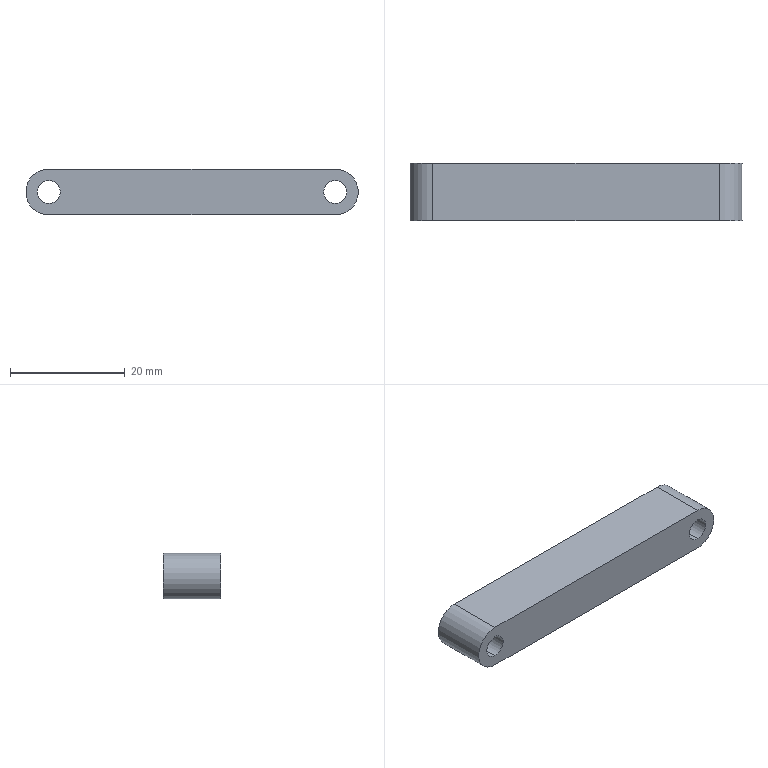Part | SolidWorks | features Extrusion 1 | 1 solid | 10 faces | box 58 x 10 x 8 mm | volume 4251 mm3 | cylinder 6 | plane 4 | commonest cylinder face diameters 4 x4 8 x2
STEP:
#1=CARTESIAN_POINT('',(25.,10.,-2.));
#2=VERTEX_POINT('',#1);
#3=CARTESIAN_POINT('',(25.,10.,2.));
#4=VERTEX_POINT('',#3);
#5=CARTESIAN_POINT('',(25.,10.,0.));
#6=DIRECTION('',(0.,1.,0.));
#7=DIRECTION('',(0.,0.,1.));
#8=AXIS2_PLACEMENT_3D('',#5,#6,#7);
#9=CIRCLE('',#8,2.);
#10=EDGE_CURVE('',#2,#4,#9,.T.);
#11=ORIENTED_EDGE('',*,*,#10,.T.);
#12=CARTESIAN_POINT('',(25.,0.,2.));
#13=VERTEX_POINT('',#12);
#14=CARTESIAN_POINT('',(25.,10.,2.));
#15=DIRECTION('',(0.,-1.,0.));
#16=VECTOR('',#15,1000.);
#17=LINE('',#14,#16);
#18=EDGE_CURVE('',#4,#13,#17,.T.);
#19=ORIENTED_EDGE('',*,*,#18,.T.);
#20=CARTESIAN_POINT('',(25.,0.,-2.));
#21=VERTEX_POINT('',#20);
#22=CARTESIAN_POINT('',(25.,0.,0.));
#23=DIRECTION('',(0.,1.,0.));
#24=DIRECTION('',(0.,0.,1.));
#25=AXIS2_PLACEMENT_3D('',#22,#23,#24);
#26=CIRCLE('',#25,2.);
#27=EDGE_CURVE('',#21,#13,#26,.T.);
#28=ORIENTED_EDGE('',*,*,#27,.F.);
#29=CARTESIAN_POINT('',(25.,10.,-2.));
#30=DIRECTION('',(0.,-1.,0.));
#31=VECTOR('',#30,1000.);
#32=LINE('',#29,#31);
#33=EDGE_CURVE('',#2,#21,#32,.T.);
#34=ORIENTED_EDGE('',*,*,#33,.F.);
#35=EDGE_LOOP('',(#11,#19,#28,#34));
#36=FACE_OUTER_BOUND('',#35,.T.);
#37=CARTESIAN_POINT('',(25.,10.,0.));
#38=DIRECTION('',(0.,-1.,0.));
#39=DIRECTION('',(0.,0.,-1.));
#40=AXIS2_PLACEMENT_3D('',#37,#38,#39);
#41=CYLINDRICAL_SURFACE('',#40,2.);
#42=ADVANCED_FACE('',(#36),#41,.F.);
#43=CARTESIAN_POINT('',(-25.,10.,-2.));
#44=VERTEX_POINT('',#43);
#45=CARTESIAN_POINT('',(-25.,10.,2.));
#46=VERTEX_POINT('',#45);
#47=CARTESIAN_POINT('',(-25.,10.,0.));
#48=DIRECTION('',(0.,1.,0.));
#49=DIRECTION('',(0.,0.,1.));
#50=AXIS2_PLACEMENT_3D('',#47,#48,#49);
#51=CIRCLE('',#50,2.);
#52=EDGE_CURVE('',#44,#46,#51,.T.);
#53=ORIENTED_EDGE('',*,*,#52,.T.);
#54=CARTESIAN_POINT('',(-25.,0.,2.));
#55=VERTEX_POINT('',#54);
#56=CARTESIAN_POINT('',(-25.,10.,2.));
#57=DIRECTION('',(0.,-1.,0.));
#58=VECTOR('',#57,1000.);
#59=LINE('',#56,#58);
#60=EDGE_CURVE('',#46,#55,#59,.T.);
#61=ORIENTED_EDGE('',*,*,#60,.T.);
#62=CARTESIAN_POINT('',(-25.,0.,-2.));
#63=VERTEX_POINT('',#62);
#64=CARTESIAN_POINT('',(-25.,0.,0.));
#65=DIRECTION('',(0.,1.,0.));
#66=DIRECTION('',(0.,0.,1.));
#67=AXIS2_PLACEMENT_3D('',#64,#65,#66);
#68=CIRCLE('',#67,2.);
#69=EDGE_CURVE('',#63,#55,#68,.T.);
#70=ORIENTED_EDGE('',*,*,#69,.F.);
#71=CARTESIAN_POINT('',(-25.,10.,-2.));
#72=DIRECTION('',(0.,-1.,0.));
#73=VECTOR('',#72,1000.);
#74=LINE('',#71,#73);
#75=EDGE_CURVE('',#44,#63,#74,.T.);
#76=ORIENTED_EDGE('',*,*,#75,.F.);
#77=EDGE_LOOP('',(#53,#61,#70,#76));
#78=FACE_OUTER_BOUND('',#77,.T.);
#79=CARTESIAN_POINT('',(-25.,10.,0.));
#80=DIRECTION('',(0.,-1.,0.));
#81=DIRECTION('',(0.,0.,-1.));
#82=AXIS2_PLACEMENT_3D('',#79,#80,#81);
#83=CYLINDRICAL_SURFACE('',#82,2.);
#84=ADVANCED_FACE('',(#78),#83,.F.);
#85=CARTESIAN_POINT('',(25.,0.,4.));
#86=VERTEX_POINT('',#85);
#87=CARTESIAN_POINT('',(-25.,0.,4.));
#88=VERTEX_POINT('',#87);
#89=CARTESIAN_POINT('',(0.,0.,4.));
#90=DIRECTION('',(-1.,0.,0.));
#91=VECTOR('',#90,1000.);
#92=LINE('',#89,#91);
#93=EDGE_CURVE('',#86,#88,#92,.T.);
#94=ORIENTED_EDGE('',*,*,#93,.F.);
#95=CARTESIAN_POINT('',(25.,10.,4.));
#96=VERTEX_POINT('',#95);
#97=CARTESIAN_POINT('',(25.,10.,4.));
#98=DIRECTION('',(0.,-1.,0.));
#99=VECTOR('',#98,1000.);
#100=LINE('',#97,#99);
#101=EDGE_CURVE('',#96,#86,#100,.T.);
#102=ORIENTED_EDGE('',*,*,#101,.F.);
#103=CARTESIAN_POINT('',(-25.,10.,4.));
#104=VERTEX_POINT('',#103);
#105=CARTESIAN_POINT('',(0.,10.,4.));
#106=DIRECTION('',(-1.,0.,0.));
#107=VECTOR('',#106,1000.);
#108=LINE('',#105,#107);
#109=EDGE_CURVE('',#96,#104,#108,.T.);
#110=ORIENTED_EDGE('',*,*,#109,.T.);
#111=CARTESIAN_POINT('',(-25.,10.,4.));
#112=DIRECTION('',(0.,-1.,0.));
#113=VECTOR('',#112,1000.);
#114=LINE('',#111,#113);
#115=EDGE_CURVE('',#104,#88,#114,.T.);
#116=ORIENTED_EDGE('',*,*,#115,.T.);
#117=EDGE_LOOP('',(#94,#102,#110,#116));
#118=FACE_OUTER_BOUND('',#117,.T.);
#119=CARTESIAN_POINT('',(0.,10.,4.));
#120=DIRECTION('',(0.,0.,1.));
#121=DIRECTION('',(1.,0.,0.));
#122=AXIS2_PLACEMENT_3D('',#119,#120,#121);
#123=PLANE('',#122);
#124=ADVANCED_FACE('',(#118),#123,.T.);
#125=CARTESIAN_POINT('',(25.,0.,-4.));
#126=VERTEX_POINT('',#125);
#127=CARTESIAN_POINT('',(25.,0.,0.));
#128=DIRECTION('',(0.,-1.,0.));
#129=DIRECTION('',(0.,0.,1.));
#130=AXIS2_PLACEMENT_3D('',#127,#128,#129);
#131=CIRCLE('',#130,4.);
#132=EDGE_CURVE('',#126,#86,#131,.T.);
#133=ORIENTED_EDGE('',*,*,#132,.F.);
#134=CARTESIAN_POINT('',(25.,10.,-4.));
#135=VERTEX_POINT('',#134);
#136=CARTESIAN_POINT('',(25.,10.,-4.));
#137=DIRECTION('',(0.,-1.,0.));
#138=VECTOR('',#137,1000.);
#139=LINE('',#136,#138);
#140=EDGE_CURVE('',#135,#126,#139,.T.);
#141=ORIENTED_EDGE('',*,*,#140,.F.);
#142=CARTESIAN_POINT('',(25.,10.,0.));
#143=DIRECTION('',(0.,-1.,0.));
#144=DIRECTION('',(0.,0.,1.));
#145=AXIS2_PLACEMENT_3D('',#142,#143,#144);
#146=CIRCLE('',#145,4.);
#147=EDGE_CURVE('',#135,#96,#146,.T.);
#148=ORIENTED_EDGE('',*,*,#147,.T.);
#149=ORIENTED_EDGE('',*,*,#101,.T.);
#150=EDGE_LOOP('',(#133,#141,#148,#149));
#151=FACE_OUTER_BOUND('',#150,.T.);
#152=CARTESIAN_POINT('',(25.,10.,0.));
#153=DIRECTION('',(0.,-1.,0.));
#154=DIRECTION('',(0.,0.,-1.));
#155=AXIS2_PLACEMENT_3D('',#152,#153,#154);
#156=CYLINDRICAL_SURFACE('',#155,4.);
#157=ADVANCED_FACE('',(#151),#156,.T.);
#158=CARTESIAN_POINT('',(-25.,0.,-4.));
#159=VERTEX_POINT('',#158);
#160=CARTESIAN_POINT('',(0.,0.,-4.));
#161=DIRECTION('',(1.,0.,0.));
#162=VECTOR('',#161,1000.);
#163=LINE('',#160,#162);
#164=EDGE_CURVE('',#159,#126,#163,.T.);
#165=ORIENTED_EDGE('',*,*,#164,.F.);
#166=CARTESIAN_POINT('',(-25.,10.,-4.));
#167=VERTEX_POINT('',#166);
#168=CARTESIAN_POINT('',(-25.,10.,-4.));
#169=DIRECTION('',(0.,-1.,0.));
#170=VECTOR('',#169,1000.);
#171=LINE('',#168,#170);
#172=EDGE_CURVE('',#167,#159,#171,.T.);
#173=ORIENTED_EDGE('',*,*,#172,.F.);
#174=CARTESIAN_POINT('',(0.,10.,-4.));
#175=DIRECTION('',(1.,0.,0.));
#176=VECTOR('',#175,1000.);
#177=LINE('',#174,#176);
#178=EDGE_CURVE('',#167,#135,#177,.T.);
#179=ORIENTED_EDGE('',*,*,#178,.T.);
#180=ORIENTED_EDGE('',*,*,#140,.T.);
#181=EDGE_LOOP('',(#165,#173,#179,#180));
#182=FACE_OUTER_BOUND('',#181,.T.);
#183=CARTESIAN_POINT('',(0.,10.,-4.));
#184=DIRECTION('',(0.,0.,-1.));
#185=DIRECTION('',(-1.,0.,0.));
#186=AXIS2_PLACEMENT_3D('',#183,#184,#185);
#187=PLANE('',#186);
#188=ADVANCED_FACE('',(#182),#187,.T.);
#189=ORIENTED_EDGE('',*,*,#60,.F.);
#190=CARTESIAN_POINT('',(-25.,10.,0.));
#191=DIRECTION('',(0.,1.,0.));
#192=DIRECTION('',(0.,0.,1.));
#193=AXIS2_PLACEMENT_3D('',#190,#191,#192);
#194=CIRCLE('',#193,2.);
#195=EDGE_CURVE('',#46,#44,#194,.T.);
#196=ORIENTED_EDGE('',*,*,#195,.T.);
#197=ORIENTED_EDGE('',*,*,#75,.T.);
#198=CARTESIAN_POINT('',(-25.,0.,0.));
#199=DIRECTION('',(0.,1.,0.));
#200=DIRECTION('',(0.,0.,1.));
#201=AXIS2_PLACEMENT_3D('',#198,#199,#200);
#202=CIRCLE('',#201,2.);
#203=EDGE_CURVE('',#55,#63,#202,.T.);
#204=ORIENTED_EDGE('',*,*,#203,.F.);
#205=EDGE_LOOP('',(#189,#196,#197,#204));
#206=FACE_OUTER_BOUND('',#205,.T.);
#207=CARTESIAN_POINT('',(-25.,10.,0.));
#208=DIRECTION('',(0.,-1.,0.));
#209=DIRECTION('',(0.,0.,-1.));
#210=AXIS2_PLACEMENT_3D('',#207,#208,#209);
#211=CYLINDRICAL_SURFACE('',#210,2.);
#212=ADVANCED_FACE('',(#206),#211,.F.);
#213=CARTESIAN_POINT('',(-25.,0.,0.));
#214=DIRECTION('',(0.,-1.,0.));
#215=DIRECTION('',(0.,0.,1.));
#216=AXIS2_PLACEMENT_3D('',#213,#214,#215);
#217=CIRCLE('',#216,4.);
#218=EDGE_CURVE('',#88,#159,#217,.T.);
#219=ORIENTED_EDGE('',*,*,#218,.F.);
#220=ORIENTED_EDGE('',*,*,#115,.F.);
#221=CARTESIAN_POINT('',(-25.,10.,0.));
#222=DIRECTION('',(0.,-1.,0.));
#223=DIRECTION('',(0.,0.,1.));
#224=AXIS2_PLACEMENT_3D('',#221,#222,#223);
#225=CIRCLE('',#224,4.);
#226=EDGE_CURVE('',#104,#167,#225,.T.);
#227=ORIENTED_EDGE('',*,*,#226,.T.);
#228=ORIENTED_EDGE('',*,*,#172,.T.);
#229=EDGE_LOOP('',(#219,#220,#227,#228));
#230=FACE_OUTER_BOUND('',#229,.T.);
#231=CARTESIAN_POINT('',(-25.,10.,0.));
#232=DIRECTION('',(0.,-1.,0.));
#233=DIRECTION('',(0.,0.,-1.));
#234=AXIS2_PLACEMENT_3D('',#231,#232,#233);
#235=CYLINDRICAL_SURFACE('',#234,4.);
#236=ADVANCED_FACE('',(#230),#235,.T.);
#237=ORIENTED_EDGE('',*,*,#18,.F.);
#238=CARTESIAN_POINT('',(25.,10.,0.));
#239=DIRECTION('',(0.,1.,0.));
#240=DIRECTION('',(0.,0.,1.));
#241=AXIS2_PLACEMENT_3D('',#238,#239,#240);
#242=CIRCLE('',#241,2.);
#243=EDGE_CURVE('',#4,#2,#242,.T.);
#244=ORIENTED_EDGE('',*,*,#243,.T.);
#245=ORIENTED_EDGE('',*,*,#33,.T.);
#246=CARTESIAN_POINT('',(25.,0.,0.));
#247=DIRECTION('',(0.,1.,0.));
#248=DIRECTION('',(0.,0.,1.));
#249=AXIS2_PLACEMENT_3D('',#246,#247,#248);
#250=CIRCLE('',#249,2.);
#251=EDGE_CURVE('',#13,#21,#250,.T.);
#252=ORIENTED_EDGE('',*,*,#251,.F.);
#253=EDGE_LOOP('',(#237,#244,#245,#252));
#254=FACE_OUTER_BOUND('',#253,.T.);
#255=CARTESIAN_POINT('',(25.,10.,0.));
#256=DIRECTION('',(0.,-1.,0.));
#257=DIRECTION('',(0.,0.,-1.));
#258=AXIS2_PLACEMENT_3D('',#255,#256,#257);
#259=CYLINDRICAL_SURFACE('',#258,2.);
#260=ADVANCED_FACE('',(#254),#259,.F.);
#261=ORIENTED_EDGE('',*,*,#109,.F.);
#262=ORIENTED_EDGE('',*,*,#147,.F.);
#263=ORIENTED_EDGE('',*,*,#178,.F.);
#264=ORIENTED_EDGE('',*,*,#226,.F.);
#265=EDGE_LOOP('',(#261,#262,#263,#264));
#266=FACE_OUTER_BOUND('',#265,.T.);
#267=ORIENTED_EDGE('',*,*,#52,.F.);
#268=ORIENTED_EDGE('',*,*,#195,.F.);
#269=EDGE_LOOP('',(#267,#268));
#270=FACE_BOUND('',#269,.T.);
#271=ORIENTED_EDGE('',*,*,#10,.F.);
#272=ORIENTED_EDGE('',*,*,#243,.F.);
#273=EDGE_LOOP('',(#271,#272));
#274=FACE_BOUND('',#273,.T.);
#275=CARTESIAN_POINT('',(0.,10.,0.));
#276=DIRECTION('',(0.,1.,0.));
#277=DIRECTION('',(0.,0.,1.));
#278=AXIS2_PLACEMENT_3D('',#275,#276,#277);
#279=PLANE('',#278);
#280=ADVANCED_FACE('',(#266,#270,#274),#279,.T.);
#281=ORIENTED_EDGE('',*,*,#93,.T.);
#282=ORIENTED_EDGE('',*,*,#218,.T.);
#283=ORIENTED_EDGE('',*,*,#164,.T.);
#284=ORIENTED_EDGE('',*,*,#132,.T.);
#285=EDGE_LOOP('',(#281,#282,#283,#284));
#286=FACE_OUTER_BOUND('',#285,.T.);
#287=ORIENTED_EDGE('',*,*,#69,.T.);
#288=ORIENTED_EDGE('',*,*,#203,.T.);
#289=EDGE_LOOP('',(#287,#288));
#290=FACE_BOUND('',#289,.T.);
#291=ORIENTED_EDGE('',*,*,#27,.T.);
#292=ORIENTED_EDGE('',*,*,#251,.T.);
#293=EDGE_LOOP('',(#291,#292));
#294=FACE_BOUND('',#293,.T.);
#295=CARTESIAN_POINT('',(0.,0.,0.));
#296=DIRECTION('',(0.,1.,0.));
#297=DIRECTION('',(0.,0.,1.));
#298=AXIS2_PLACEMENT_3D('',#295,#296,#297);
#299=PLANE('',#298);
#300=ADVANCED_FACE('',(#286,#290,#294),#299,.F.);
#301=CLOSED_SHELL('',(#42,#84,#124,#157,#188,#212,#236,#260,#280,#300));
#302=MANIFOLD_SOLID_BREP('',#301);
#303=CARTESIAN_POINT('',(0.,0.,0.));
#304=DIRECTION('',(0.,0.,1.));
#305=DIRECTION('',(1.,0.,0.));
#306=AXIS2_PLACEMENT_3D('',#303,#304,#305);
#307=(LENGTH_UNIT()NAMED_UNIT(*)SI_UNIT(.MILLI.,.METRE.));
#308=UNCERTAINTY_MEASURE_WITH_UNIT(LENGTH_MEASURE(0.00001),#307,'','');
#309=(NAMED_UNIT(*)PLANE_ANGLE_UNIT()SI_UNIT($,.RADIAN.));
#310=(NAMED_UNIT(*)SI_UNIT($,.STERADIAN.)SOLID_ANGLE_UNIT());
#311=(GEOMETRIC_REPRESENTATION_CONTEXT(3)GLOBAL_UNCERTAINTY_ASSIGNED_CONTEXT((#308))GLOBAL_UNIT_ASSIGNED_CONTEXT((#307,#309,#310))REPRESENTATION_CONTEXT('',''));
#312=ADVANCED_BREP_SHAPE_REPRESENTATION('',(#302,#306),#311);